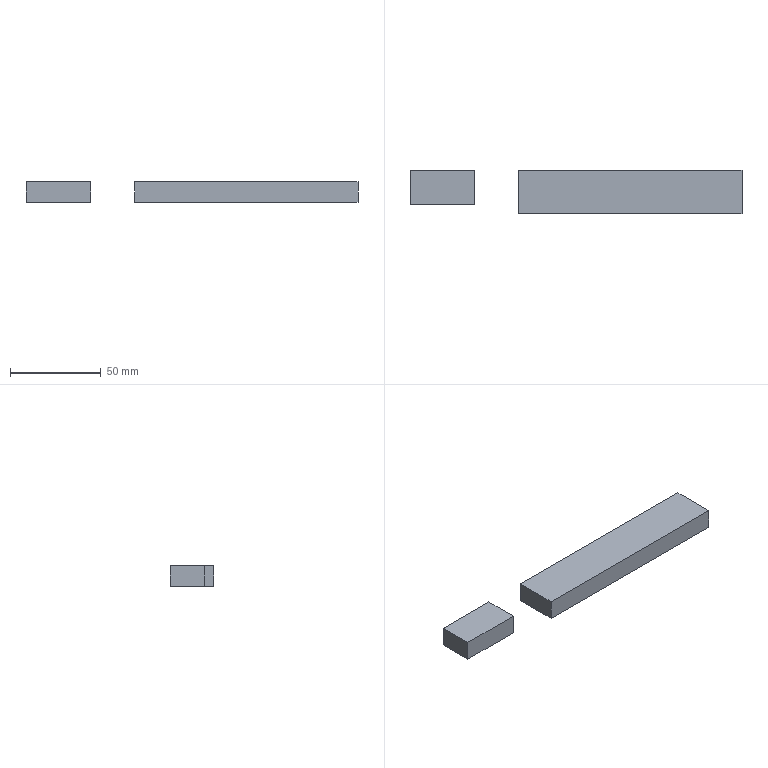Part | NX | features BREP 2 | 2 solids | 12 faces | box 182.5 x 24 x 11.2 mm | volume 40549 mm3 | plane 12
STEP:
#1=CARTESIAN_POINT('',(469.042,12.398,0.));
#2=VERTEX_POINT('',#1);
#3=CARTESIAN_POINT('',(346.442,12.398,0.));
#4=VERTEX_POINT('',#3);
#5=CARTESIAN_POINT('',(407.742,12.398,0.));
#6=DIRECTION('',(-1.,0.,0.));
#7=VECTOR('',#6,1000.);
#8=LINE('',#5,#7);
#9=EDGE_CURVE('',#2,#4,#8,.T.);
#10=ORIENTED_EDGE('',*,*,#9,.F.);
#11=CARTESIAN_POINT('',(469.042,36.398,0.));
#12=VERTEX_POINT('',#11);
#13=CARTESIAN_POINT('',(469.042,24.398,0.));
#14=DIRECTION('',(0.,-1.,0.));
#15=VECTOR('',#14,1000.);
#16=LINE('',#13,#15);
#17=EDGE_CURVE('',#12,#2,#16,.T.);
#18=ORIENTED_EDGE('',*,*,#17,.F.);
#19=CARTESIAN_POINT('',(346.442,36.398,0.));
#20=VERTEX_POINT('',#19);
#21=CARTESIAN_POINT('',(407.742,36.398,0.));
#22=DIRECTION('',(1.,0.,0.));
#23=VECTOR('',#22,1000.);
#24=LINE('',#21,#23);
#25=EDGE_CURVE('',#20,#12,#24,.T.);
#26=ORIENTED_EDGE('',*,*,#25,.F.);
#27=CARTESIAN_POINT('',(346.442,24.398,0.));
#28=DIRECTION('',(0.,1.,0.));
#29=VECTOR('',#28,1000.);
#30=LINE('',#27,#29);
#31=EDGE_CURVE('',#4,#20,#30,.T.);
#32=ORIENTED_EDGE('',*,*,#31,.F.);
#33=EDGE_LOOP('',(#10,#18,#26,#32));
#34=FACE_BOUND('',#33,.T.);
#35=CARTESIAN_POINT('',(407.742,24.398,0.));
#36=DIRECTION('',(0.,0.,1.));
#37=DIRECTION('',(-1.,0.,0.));
#38=AXIS2_PLACEMENT_3D('',#35,#36,#37);
#39=PLANE('',#38);
#40=ADVANCED_FACE('',(#34),#39,.T.);
#41=CARTESIAN_POINT('',(469.042,12.398,-11.2));
#42=VERTEX_POINT('',#41);
#43=CARTESIAN_POINT('',(469.042,12.398,-11.2));
#44=DIRECTION('',(0.,0.,1.));
#45=VECTOR('',#44,1000.);
#46=LINE('',#43,#45);
#47=EDGE_CURVE('',#42,#2,#46,.T.);
#48=ORIENTED_EDGE('',*,*,#47,.T.);
#49=ORIENTED_EDGE('',*,*,#9,.T.);
#50=CARTESIAN_POINT('',(346.442,12.398,-11.2));
#51=VERTEX_POINT('',#50);
#52=CARTESIAN_POINT('',(346.442,12.398,-11.2));
#53=DIRECTION('',(0.,0.,1.));
#54=VECTOR('',#53,1000.);
#55=LINE('',#52,#54);
#56=EDGE_CURVE('',#51,#4,#55,.T.);
#57=ORIENTED_EDGE('',*,*,#56,.F.);
#58=CARTESIAN_POINT('',(407.742,12.398,-11.2));
#59=DIRECTION('',(1.,0.,0.));
#60=VECTOR('',#59,1000.);
#61=LINE('',#58,#60);
#62=EDGE_CURVE('',#51,#42,#61,.T.);
#63=ORIENTED_EDGE('',*,*,#62,.T.);
#64=EDGE_LOOP('',(#48,#49,#57,#63));
#65=FACE_BOUND('',#64,.T.);
#66=CARTESIAN_POINT('',(407.742,12.398,-11.2));
#67=DIRECTION('',(0.,-1.,0.));
#68=DIRECTION('',(0.,0.,1.));
#69=AXIS2_PLACEMENT_3D('',#66,#67,#68);
#70=PLANE('',#69);
#71=ADVANCED_FACE('',(#65),#70,.T.);
#72=ORIENTED_EDGE('',*,*,#56,.T.);
#73=ORIENTED_EDGE('',*,*,#31,.T.);
#74=CARTESIAN_POINT('',(346.442,36.398,-11.2));
#75=VERTEX_POINT('',#74);
#76=CARTESIAN_POINT('',(346.442,36.398,-11.2));
#77=DIRECTION('',(0.,0.,1.));
#78=VECTOR('',#77,1000.);
#79=LINE('',#76,#78);
#80=EDGE_CURVE('',#75,#20,#79,.T.);
#81=ORIENTED_EDGE('',*,*,#80,.F.);
#82=CARTESIAN_POINT('',(346.442,24.398,-11.2));
#83=DIRECTION('',(0.,-1.,0.));
#84=VECTOR('',#83,1000.);
#85=LINE('',#82,#84);
#86=EDGE_CURVE('',#75,#51,#85,.T.);
#87=ORIENTED_EDGE('',*,*,#86,.T.);
#88=EDGE_LOOP('',(#72,#73,#81,#87));
#89=FACE_BOUND('',#88,.T.);
#90=CARTESIAN_POINT('',(346.442,24.398,-11.2));
#91=DIRECTION('',(-1.,0.,0.));
#92=DIRECTION('',(0.,0.,-1.));
#93=AXIS2_PLACEMENT_3D('',#90,#91,#92);
#94=PLANE('',#93);
#95=ADVANCED_FACE('',(#89),#94,.T.);
#96=ORIENTED_EDGE('',*,*,#80,.T.);
#97=ORIENTED_EDGE('',*,*,#25,.T.);
#98=CARTESIAN_POINT('',(469.042,36.398,-11.2));
#99=VERTEX_POINT('',#98);
#100=CARTESIAN_POINT('',(469.042,36.398,-11.2));
#101=DIRECTION('',(0.,0.,1.));
#102=VECTOR('',#101,1000.);
#103=LINE('',#100,#102);
#104=EDGE_CURVE('',#99,#12,#103,.T.);
#105=ORIENTED_EDGE('',*,*,#104,.F.);
#106=CARTESIAN_POINT('',(407.742,36.398,-11.2));
#107=DIRECTION('',(-1.,0.,0.));
#108=VECTOR('',#107,1000.);
#109=LINE('',#106,#108);
#110=EDGE_CURVE('',#99,#75,#109,.T.);
#111=ORIENTED_EDGE('',*,*,#110,.T.);
#112=EDGE_LOOP('',(#96,#97,#105,#111));
#113=FACE_BOUND('',#112,.T.);
#114=CARTESIAN_POINT('',(407.742,36.398,-11.2));
#115=DIRECTION('',(0.,1.,0.));
#116=DIRECTION('',(0.,0.,-1.));
#117=AXIS2_PLACEMENT_3D('',#114,#115,#116);
#118=PLANE('',#117);
#119=ADVANCED_FACE('',(#113),#118,.T.);
#120=CARTESIAN_POINT('',(469.042,24.398,-11.2));
#121=DIRECTION('',(0.,1.,0.));
#122=VECTOR('',#121,1000.);
#123=LINE('',#120,#122);
#124=EDGE_CURVE('',#42,#99,#123,.T.);
#125=ORIENTED_EDGE('',*,*,#124,.F.);
#126=ORIENTED_EDGE('',*,*,#62,.F.);
#127=ORIENTED_EDGE('',*,*,#86,.F.);
#128=ORIENTED_EDGE('',*,*,#110,.F.);
#129=EDGE_LOOP('',(#125,#126,#127,#128));
#130=FACE_BOUND('',#129,.T.);
#131=CARTESIAN_POINT('',(407.742,24.398,-11.2));
#132=DIRECTION('',(0.,0.,-1.));
#133=DIRECTION('',(1.,0.,0.));
#134=AXIS2_PLACEMENT_3D('',#131,#132,#133);
#135=PLANE('',#134);
#136=ADVANCED_FACE('',(#130),#135,.T.);
#137=ORIENTED_EDGE('',*,*,#124,.T.);
#138=ORIENTED_EDGE('',*,*,#104,.T.);
#139=ORIENTED_EDGE('',*,*,#17,.T.);
#140=ORIENTED_EDGE('',*,*,#47,.F.);
#141=EDGE_LOOP('',(#137,#138,#139,#140));
#142=FACE_BOUND('',#141,.T.);
#143=CARTESIAN_POINT('',(469.042,24.398,-11.2));
#144=DIRECTION('',(1.,0.,0.));
#145=DIRECTION('',(0.,0.,1.));
#146=AXIS2_PLACEMENT_3D('',#143,#144,#145);
#147=PLANE('',#146);
#148=ADVANCED_FACE('',(#142),#147,.T.);
#149=CLOSED_SHELL('',(#40,#71,#95,#119,#136,#148));
#150=MANIFOLD_SOLID_BREP('',#149);
#151=CARTESIAN_POINT('',(322.042,17.298,0.));
#152=VERTEX_POINT('',#151);
#153=CARTESIAN_POINT('',(286.542,17.298,0.));
#154=VERTEX_POINT('',#153);
#155=CARTESIAN_POINT('',(304.292,17.298,0.));
#156=DIRECTION('',(-1.,0.,0.));
#157=VECTOR('',#156,1000.);
#158=LINE('',#155,#157);
#159=EDGE_CURVE('',#152,#154,#158,.T.);
#160=ORIENTED_EDGE('',*,*,#159,.F.);
#161=CARTESIAN_POINT('',(322.042,36.398,0.));
#162=VERTEX_POINT('',#161);
#163=CARTESIAN_POINT('',(322.042,26.848,0.));
#164=DIRECTION('',(0.,-1.,0.));
#165=VECTOR('',#164,1000.);
#166=LINE('',#163,#165);
#167=EDGE_CURVE('',#162,#152,#166,.T.);
#168=ORIENTED_EDGE('',*,*,#167,.F.);
#169=CARTESIAN_POINT('',(286.542,36.398,0.));
#170=VERTEX_POINT('',#169);
#171=CARTESIAN_POINT('',(304.292,36.398,0.));
#172=DIRECTION('',(1.,0.,0.));
#173=VECTOR('',#172,1000.);
#174=LINE('',#171,#173);
#175=EDGE_CURVE('',#170,#162,#174,.T.);
#176=ORIENTED_EDGE('',*,*,#175,.F.);
#177=CARTESIAN_POINT('',(286.542,26.848,0.));
#178=DIRECTION('',(0.,1.,0.));
#179=VECTOR('',#178,1000.);
#180=LINE('',#177,#179);
#181=EDGE_CURVE('',#154,#170,#180,.T.);
#182=ORIENTED_EDGE('',*,*,#181,.F.);
#183=EDGE_LOOP('',(#160,#168,#176,#182));
#184=FACE_BOUND('',#183,.T.);
#185=CARTESIAN_POINT('',(304.292,26.848,0.));
#186=DIRECTION('',(0.,0.,1.));
#187=DIRECTION('',(-1.,0.,0.));
#188=AXIS2_PLACEMENT_3D('',#185,#186,#187);
#189=PLANE('',#188);
#190=ADVANCED_FACE('',(#184),#189,.T.);
#191=CARTESIAN_POINT('',(322.042,17.298,-11.2));
#192=VERTEX_POINT('',#191);
#193=CARTESIAN_POINT('',(322.042,17.298,-11.2));
#194=DIRECTION('',(0.,0.,1.));
#195=VECTOR('',#194,1000.);
#196=LINE('',#193,#195);
#197=EDGE_CURVE('',#192,#152,#196,.T.);
#198=ORIENTED_EDGE('',*,*,#197,.T.);
#199=ORIENTED_EDGE('',*,*,#159,.T.);
#200=CARTESIAN_POINT('',(286.542,17.298,-11.2));
#201=VERTEX_POINT('',#200);
#202=CARTESIAN_POINT('',(286.542,17.298,-11.2));
#203=DIRECTION('',(0.,0.,1.));
#204=VECTOR('',#203,1000.);
#205=LINE('',#202,#204);
#206=EDGE_CURVE('',#201,#154,#205,.T.);
#207=ORIENTED_EDGE('',*,*,#206,.F.);
#208=CARTESIAN_POINT('',(304.292,17.298,-11.2));
#209=DIRECTION('',(1.,0.,0.));
#210=VECTOR('',#209,1000.);
#211=LINE('',#208,#210);
#212=EDGE_CURVE('',#201,#192,#211,.T.);
#213=ORIENTED_EDGE('',*,*,#212,.T.);
#214=EDGE_LOOP('',(#198,#199,#207,#213));
#215=FACE_BOUND('',#214,.T.);
#216=CARTESIAN_POINT('',(304.292,17.298,-11.2));
#217=DIRECTION('',(0.,-1.,0.));
#218=DIRECTION('',(0.,0.,1.));
#219=AXIS2_PLACEMENT_3D('',#216,#217,#218);
#220=PLANE('',#219);
#221=ADVANCED_FACE('',(#215),#220,.T.);
#222=ORIENTED_EDGE('',*,*,#206,.T.);
#223=ORIENTED_EDGE('',*,*,#181,.T.);
#224=CARTESIAN_POINT('',(286.542,36.398,-11.2));
#225=VERTEX_POINT('',#224);
#226=CARTESIAN_POINT('',(286.542,36.398,-11.2));
#227=DIRECTION('',(0.,0.,1.));
#228=VECTOR('',#227,1000.);
#229=LINE('',#226,#228);
#230=EDGE_CURVE('',#225,#170,#229,.T.);
#231=ORIENTED_EDGE('',*,*,#230,.F.);
#232=CARTESIAN_POINT('',(286.542,26.848,-11.2));
#233=DIRECTION('',(0.,-1.,0.));
#234=VECTOR('',#233,1000.);
#235=LINE('',#232,#234);
#236=EDGE_CURVE('',#225,#201,#235,.T.);
#237=ORIENTED_EDGE('',*,*,#236,.T.);
#238=EDGE_LOOP('',(#222,#223,#231,#237));
#239=FACE_BOUND('',#238,.T.);
#240=CARTESIAN_POINT('',(286.542,26.848,-11.2));
#241=DIRECTION('',(-1.,0.,0.));
#242=DIRECTION('',(0.,0.,-1.));
#243=AXIS2_PLACEMENT_3D('',#240,#241,#242);
#244=PLANE('',#243);
#245=ADVANCED_FACE('',(#239),#244,.T.);
#246=ORIENTED_EDGE('',*,*,#230,.T.);
#247=ORIENTED_EDGE('',*,*,#175,.T.);
#248=CARTESIAN_POINT('',(322.042,36.398,-11.2));
#249=VERTEX_POINT('',#248);
#250=CARTESIAN_POINT('',(322.042,36.398,-11.2));
#251=DIRECTION('',(0.,0.,1.));
#252=VECTOR('',#251,1000.);
#253=LINE('',#250,#252);
#254=EDGE_CURVE('',#249,#162,#253,.T.);
#255=ORIENTED_EDGE('',*,*,#254,.F.);
#256=CARTESIAN_POINT('',(304.292,36.398,-11.2));
#257=DIRECTION('',(-1.,0.,0.));
#258=VECTOR('',#257,1000.);
#259=LINE('',#256,#258);
#260=EDGE_CURVE('',#249,#225,#259,.T.);
#261=ORIENTED_EDGE('',*,*,#260,.T.);
#262=EDGE_LOOP('',(#246,#247,#255,#261));
#263=FACE_BOUND('',#262,.T.);
#264=CARTESIAN_POINT('',(304.292,36.398,-11.2));
#265=DIRECTION('',(0.,1.,0.));
#266=DIRECTION('',(0.,0.,-1.));
#267=AXIS2_PLACEMENT_3D('',#264,#265,#266);
#268=PLANE('',#267);
#269=ADVANCED_FACE('',(#263),#268,.T.);
#270=CARTESIAN_POINT('',(322.042,26.848,-11.2));
#271=DIRECTION('',(0.,1.,0.));
#272=VECTOR('',#271,1000.);
#273=LINE('',#270,#272);
#274=EDGE_CURVE('',#192,#249,#273,.T.);
#275=ORIENTED_EDGE('',*,*,#274,.F.);
#276=ORIENTED_EDGE('',*,*,#212,.F.);
#277=ORIENTED_EDGE('',*,*,#236,.F.);
#278=ORIENTED_EDGE('',*,*,#260,.F.);
#279=EDGE_LOOP('',(#275,#276,#277,#278));
#280=FACE_BOUND('',#279,.T.);
#281=CARTESIAN_POINT('',(304.292,26.848,-11.2));
#282=DIRECTION('',(0.,0.,-1.));
#283=DIRECTION('',(1.,0.,0.));
#284=AXIS2_PLACEMENT_3D('',#281,#282,#283);
#285=PLANE('',#284);
#286=ADVANCED_FACE('',(#280),#285,.T.);
#287=ORIENTED_EDGE('',*,*,#274,.T.);
#288=ORIENTED_EDGE('',*,*,#254,.T.);
#289=ORIENTED_EDGE('',*,*,#167,.T.);
#290=ORIENTED_EDGE('',*,*,#197,.F.);
#291=EDGE_LOOP('',(#287,#288,#289,#290));
#292=FACE_BOUND('',#291,.T.);
#293=CARTESIAN_POINT('',(322.042,26.848,-11.2));
#294=DIRECTION('',(1.,0.,0.));
#295=DIRECTION('',(0.,0.,1.));
#296=AXIS2_PLACEMENT_3D('',#293,#294,#295);
#297=PLANE('',#296);
#298=ADVANCED_FACE('',(#292),#297,.T.);
#299=CLOSED_SHELL('',(#190,#221,#245,#269,#286,#298));
#300=MANIFOLD_SOLID_BREP('',#299);
#301=(LENGTH_UNIT()NAMED_UNIT(*)SI_UNIT(.MILLI.,.METRE.));
#302=UNCERTAINTY_MEASURE_WITH_UNIT(LENGTH_MEASURE(0.00001),#301,'','');
#303=(NAMED_UNIT(*)PLANE_ANGLE_UNIT()SI_UNIT($,.RADIAN.));
#304=(NAMED_UNIT(*)SI_UNIT($,.STERADIAN.)SOLID_ANGLE_UNIT());
#305=(GEOMETRIC_REPRESENTATION_CONTEXT(3)GLOBAL_UNCERTAINTY_ASSIGNED_CONTEXT((#302))GLOBAL_UNIT_ASSIGNED_CONTEXT((#301,#303,#304))REPRESENTATION_CONTEXT('',''));
#306=ADVANCED_BREP_SHAPE_REPRESENTATION('',(#150,#300),#305);